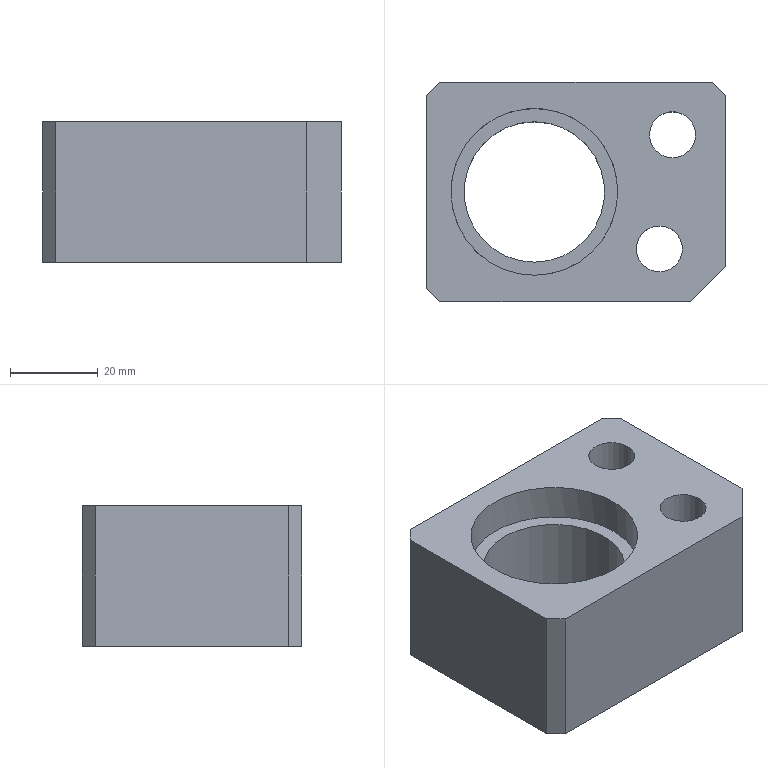Part | STEP file | lll_id3594_x_t | 1 solid | 19 faces | box 68 x 50 x 32 mm | volume 68588 mm3 | plane 13 | cylinder 6 | commonest cylinder face diameters 10.5 x2 17 x2 32 x1 38 x1
STEP:
#1=CARTESIAN_POINT('',(3231.727,69.288,77.5));
#2=VERTEX_POINT('',#1);
#3=CARTESIAN_POINT('',(3236.977,69.288,77.5));
#4=DIRECTION('',(0.,0.,1.));
#5=DIRECTION('',(-1.,0.,0.));
#6=AXIS2_PLACEMENT_3D('',#3,#4,#5);
#7=CIRCLE('',#6,5.25);
#8=EDGE_CURVE('',#2,#2,#7,.T.);
#9=ORIENTED_EDGE('',*,*,#8,.T.);
#10=EDGE_LOOP('',(#9));
#11=FACE_BOUND('',#10,.T.);
#12=CARTESIAN_POINT('',(3228.477,69.288,77.5));
#13=VERTEX_POINT('',#12);
#14=CARTESIAN_POINT('',(3236.977,69.288,77.5));
#15=DIRECTION('',(0.,0.,1.));
#16=DIRECTION('',(-1.,0.,0.));
#17=AXIS2_PLACEMENT_3D('',#14,#15,#16);
#18=CIRCLE('',#17,8.5);
#19=EDGE_CURVE('',#13,#13,#18,.T.);
#20=ORIENTED_EDGE('',*,*,#19,.F.);
#21=EDGE_LOOP('',(#20));
#22=FACE_BOUND('',#21,.T.);
#23=CARTESIAN_POINT('',(3236.977,69.288,77.5));
#24=DIRECTION('',(0.,0.,1.));
#25=DIRECTION('',(0.,1.,0.));
#26=AXIS2_PLACEMENT_3D('',#23,#24,#25);
#27=PLANE('',#26);
#28=ADVANCED_FACE('',(#11,#22),#27,.F.);
#29=CARTESIAN_POINT('',(3205.477,75.288,84.3));
#30=VERTEX_POINT('',#29);
#31=CARTESIAN_POINT('',(3205.477,56.288,84.3));
#32=DIRECTION('',(0.,0.,1.));
#33=DIRECTION('',(0.,1.,0.));
#34=AXIS2_PLACEMENT_3D('',#31,#32,#33);
#35=CIRCLE('',#34,19.);
#36=EDGE_CURVE('',#30,#30,#35,.T.);
#37=ORIENTED_EDGE('',*,*,#36,.T.);
#38=EDGE_LOOP('',(#37));
#39=FACE_BOUND('',#38,.T.);
#40=CARTESIAN_POINT('',(3205.477,72.288,84.3));
#41=VERTEX_POINT('',#40);
#42=CARTESIAN_POINT('',(3205.477,56.288,84.3));
#43=DIRECTION('',(0.,0.,1.));
#44=DIRECTION('',(0.,1.,0.));
#45=AXIS2_PLACEMENT_3D('',#42,#43,#44);
#46=CIRCLE('',#45,16.);
#47=EDGE_CURVE('',#41,#41,#46,.T.);
#48=ORIENTED_EDGE('',*,*,#47,.F.);
#49=EDGE_LOOP('',(#48));
#50=FACE_BOUND('',#49,.T.);
#51=CARTESIAN_POINT('',(3214.227,56.288,84.3));
#52=DIRECTION('',(0.,0.,-1.));
#53=DIRECTION('',(1.,0.,0.));
#54=AXIS2_PLACEMENT_3D('',#51,#52,#53);
#55=PLANE('',#54);
#56=ADVANCED_FACE('',(#39,#50),#55,.F.);
#57=ORIENTED_EDGE('',*,*,#19,.T.);
#58=EDGE_LOOP('',(#57));
#59=FACE_BOUND('',#58,.T.);
#60=CARTESIAN_POINT('',(3228.477,69.288,60.5));
#61=VERTEX_POINT('',#60);
#62=CARTESIAN_POINT('',(3236.977,69.288,60.5));
#63=DIRECTION('',(0.,0.,-1.));
#64=DIRECTION('',(-1.,0.,0.));
#65=AXIS2_PLACEMENT_3D('',#62,#63,#64);
#66=CIRCLE('',#65,8.5);
#67=EDGE_CURVE('',#61,#61,#66,.T.);
#68=ORIENTED_EDGE('',*,*,#67,.T.);
#69=EDGE_LOOP('',(#68));
#70=FACE_BOUND('',#69,.T.);
#71=CARTESIAN_POINT('',(3236.977,69.288,60.5));
#72=DIRECTION('',(0.,0.,1.));
#73=DIRECTION('',(0.,1.,0.));
#74=AXIS2_PLACEMENT_3D('',#71,#72,#73);
#75=CYLINDRICAL_SURFACE('',#74,8.5);
#76=ADVANCED_FACE('',(#59,#70),#75,.F.);
#77=CARTESIAN_POINT('',(3183.977,31.288,60.5));
#78=VERTEX_POINT('',#77);
#79=CARTESIAN_POINT('',(3180.977,34.288,60.5));
#80=VERTEX_POINT('',#79);
#81=CARTESIAN_POINT('',(3164.794,50.47,60.5));
#82=DIRECTION('',(-0.7071,0.7071,0.));
#83=VECTOR('',#82,1.);
#84=LINE('',#81,#83);
#85=EDGE_CURVE('',#78,#80,#84,.T.);
#86=ORIENTED_EDGE('',*,*,#85,.F.);
#87=CARTESIAN_POINT('',(3183.977,31.288,92.5));
#88=VERTEX_POINT('',#87);
#89=CARTESIAN_POINT('',(3183.977,31.288,-8.5));
#90=DIRECTION('',(0.,0.,-1.));
#91=VECTOR('',#90,1.);
#92=LINE('',#89,#91);
#93=EDGE_CURVE('',#88,#78,#92,.T.);
#94=ORIENTED_EDGE('',*,*,#93,.F.);
#95=CARTESIAN_POINT('',(3180.977,34.288,92.5));
#96=VERTEX_POINT('',#95);
#97=CARTESIAN_POINT('',(3164.794,50.47,92.5));
#98=DIRECTION('',(0.7071,-0.7071,0.));
#99=VECTOR('',#98,1.);
#100=LINE('',#97,#99);
#101=EDGE_CURVE('',#96,#88,#100,.T.);
#102=ORIENTED_EDGE('',*,*,#101,.F.);
#103=CARTESIAN_POINT('',(3180.977,34.288,-8.5));
#104=DIRECTION('',(0.,0.,1.));
#105=VECTOR('',#104,1.);
#106=LINE('',#103,#105);
#107=EDGE_CURVE('',#80,#96,#106,.T.);
#108=ORIENTED_EDGE('',*,*,#107,.F.);
#109=EDGE_LOOP('',(#86,#94,#102,#108));
#110=FACE_OUTER_BOUND('',#109,.T.);
#111=CARTESIAN_POINT('',(3180.977,34.288,-8.5));
#112=DIRECTION('',(0.7071,0.7071,0.));
#113=DIRECTION('',(0.,0.,1.));
#114=AXIS2_PLACEMENT_3D('',#111,#112,#113);
#115=PLANE('',#114);
#116=ADVANCED_FACE('',(#110),#115,.F.);
#117=CARTESIAN_POINT('',(3180.977,78.288,60.5));
#118=VERTEX_POINT('',#117);
#119=CARTESIAN_POINT('',(3180.977,119.478,60.5));
#120=DIRECTION('',(0.,1.,0.));
#121=VECTOR('',#120,1.);
#122=LINE('',#119,#121);
#123=EDGE_CURVE('',#80,#118,#122,.T.);
#124=ORIENTED_EDGE('',*,*,#123,.F.);
#125=ORIENTED_EDGE('',*,*,#107,.T.);
#126=CARTESIAN_POINT('',(3180.977,78.288,92.5));
#127=VERTEX_POINT('',#126);
#128=CARTESIAN_POINT('',(3180.977,56.288,92.5));
#129=DIRECTION('',(0.,-1.,0.));
#130=VECTOR('',#129,1.);
#131=LINE('',#128,#130);
#132=EDGE_CURVE('',#127,#96,#131,.T.);
#133=ORIENTED_EDGE('',*,*,#132,.F.);
#134=CARTESIAN_POINT('',(3180.977,78.288,-8.5));
#135=DIRECTION('',(0.,0.,1.));
#136=VECTOR('',#135,1.);
#137=LINE('',#134,#136);
#138=EDGE_CURVE('',#118,#127,#137,.T.);
#139=ORIENTED_EDGE('',*,*,#138,.F.);
#140=EDGE_LOOP('',(#124,#125,#133,#139));
#141=FACE_OUTER_BOUND('',#140,.T.);
#142=CARTESIAN_POINT('',(3180.977,56.288,-8.5));
#143=DIRECTION('',(-1.,0.,0.));
#144=DIRECTION('',(0.,0.,-1.));
#145=AXIS2_PLACEMENT_3D('',#142,#143,#144);
#146=PLANE('',#145);
#147=ADVANCED_FACE('',(#141),#146,.T.);
#148=CARTESIAN_POINT('',(3183.977,81.288,92.5));
#149=VERTEX_POINT('',#148);
#150=CARTESIAN_POINT('',(3183.977,81.288,92.5));
#151=DIRECTION('',(0.7071,0.7071,0.));
#152=VECTOR('',#151,1.);
#153=LINE('',#150,#152);
#154=EDGE_CURVE('',#127,#149,#153,.T.);
#155=ORIENTED_EDGE('',*,*,#154,.T.);
#156=CARTESIAN_POINT('',(3183.977,81.288,60.5));
#157=VERTEX_POINT('',#156);
#158=CARTESIAN_POINT('',(3183.977,81.288,-8.5));
#159=DIRECTION('',(0.,0.,-1.));
#160=VECTOR('',#159,1.);
#161=LINE('',#158,#160);
#162=EDGE_CURVE('',#149,#157,#161,.T.);
#163=ORIENTED_EDGE('',*,*,#162,.T.);
#164=CARTESIAN_POINT('',(3179.027,76.338,60.5));
#165=DIRECTION('',(-0.7071,-0.7071,0.));
#166=VECTOR('',#165,1.);
#167=LINE('',#164,#166);
#168=EDGE_CURVE('',#157,#118,#167,.T.);
#169=ORIENTED_EDGE('',*,*,#168,.T.);
#170=ORIENTED_EDGE('',*,*,#138,.T.);
#171=EDGE_LOOP('',(#155,#163,#169,#170));
#172=FACE_OUTER_BOUND('',#171,.T.);
#173=CARTESIAN_POINT('',(3183.977,81.288,-8.5));
#174=DIRECTION('',(0.7071,-0.7071,0.));
#175=DIRECTION('',(0.7071,0.7071,0.));
#176=AXIS2_PLACEMENT_3D('',#173,#174,#175);
#177=PLANE('',#176);
#178=ADVANCED_FACE('',(#172),#177,.F.);
#179=CARTESIAN_POINT('',(3245.977,81.288,60.5));
#180=VERTEX_POINT('',#179);
#181=CARTESIAN_POINT('',(3231.752,81.288,60.5));
#182=DIRECTION('',(1.,0.,0.));
#183=VECTOR('',#182,1.);
#184=LINE('',#181,#183);
#185=EDGE_CURVE('',#157,#180,#184,.T.);
#186=ORIENTED_EDGE('',*,*,#185,.F.);
#187=ORIENTED_EDGE('',*,*,#162,.F.);
#188=CARTESIAN_POINT('',(3245.977,81.288,92.5));
#189=VERTEX_POINT('',#188);
#190=CARTESIAN_POINT('',(3236.702,81.288,92.5));
#191=DIRECTION('',(-1.,0.,0.));
#192=VECTOR('',#191,1.);
#193=LINE('',#190,#192);
#194=EDGE_CURVE('',#189,#149,#193,.T.);
#195=ORIENTED_EDGE('',*,*,#194,.F.);
#196=CARTESIAN_POINT('',(3245.977,81.288,-8.5));
#197=DIRECTION('',(0.,0.,1.));
#198=VECTOR('',#197,1.);
#199=LINE('',#196,#198);
#200=EDGE_CURVE('',#180,#189,#199,.T.);
#201=ORIENTED_EDGE('',*,*,#200,.F.);
#202=EDGE_LOOP('',(#186,#187,#195,#201));
#203=FACE_OUTER_BOUND('',#202,.T.);
#204=CARTESIAN_POINT('',(3205.477,81.288,-8.5));
#205=DIRECTION('',(0.,1.,0.));
#206=DIRECTION('',(0.,0.,-1.));
#207=AXIS2_PLACEMENT_3D('',#204,#205,#206);
#208=PLANE('',#207);
#209=ADVANCED_FACE('',(#203),#208,.T.);
#210=CARTESIAN_POINT('',(3248.977,78.288,92.5));
#211=VERTEX_POINT('',#210);
#212=CARTESIAN_POINT('',(3248.977,78.288,92.5));
#213=DIRECTION('',(0.7071,-0.7071,0.));
#214=VECTOR('',#213,1.);
#215=LINE('',#212,#214);
#216=EDGE_CURVE('',#189,#211,#215,.T.);
#217=ORIENTED_EDGE('',*,*,#216,.T.);
#218=CARTESIAN_POINT('',(3248.977,78.288,60.5));
#219=VERTEX_POINT('',#218);
#220=CARTESIAN_POINT('',(3248.977,78.288,-8.5));
#221=DIRECTION('',(0.,0.,-1.));
#222=VECTOR('',#221,1.);
#223=LINE('',#220,#222);
#224=EDGE_CURVE('',#211,#219,#223,.T.);
#225=ORIENTED_EDGE('',*,*,#224,.T.);
#226=CARTESIAN_POINT('',(3248.977,78.288,60.5));
#227=DIRECTION('',(-0.7071,0.7071,0.));
#228=VECTOR('',#227,1.);
#229=LINE('',#226,#228);
#230=EDGE_CURVE('',#219,#180,#229,.T.);
#231=ORIENTED_EDGE('',*,*,#230,.T.);
#232=ORIENTED_EDGE('',*,*,#200,.T.);
#233=EDGE_LOOP('',(#217,#225,#231,#232));
#234=FACE_OUTER_BOUND('',#233,.T.);
#235=CARTESIAN_POINT('',(3248.977,78.288,-8.5));
#236=DIRECTION('',(-0.7071,-0.7071,0.));
#237=DIRECTION('',(0.7071,-0.7071,0.));
#238=AXIS2_PLACEMENT_3D('',#235,#236,#237);
#239=PLANE('',#238);
#240=ADVANCED_FACE('',(#234),#239,.F.);
#241=CARTESIAN_POINT('',(3248.977,39.288,92.5));
#242=VERTEX_POINT('',#241);
#243=CARTESIAN_POINT('',(3248.977,56.288,92.5));
#244=DIRECTION('',(0.,1.,0.));
#245=VECTOR('',#244,1.);
#246=LINE('',#243,#245);
#247=EDGE_CURVE('',#242,#211,#246,.T.);
#248=ORIENTED_EDGE('',*,*,#247,.F.);
#249=CARTESIAN_POINT('',(3248.977,39.288,60.5));
#250=VERTEX_POINT('',#249);
#251=CARTESIAN_POINT('',(3248.977,39.288,-8.5));
#252=DIRECTION('',(0.,0.,-1.));
#253=VECTOR('',#252,1.);
#254=LINE('',#251,#253);
#255=EDGE_CURVE('',#242,#250,#254,.T.);
#256=ORIENTED_EDGE('',*,*,#255,.T.);
#257=CARTESIAN_POINT('',(3248.977,119.478,60.5));
#258=DIRECTION('',(0.,-1.,0.));
#259=VECTOR('',#258,1.);
#260=LINE('',#257,#259);
#261=EDGE_CURVE('',#219,#250,#260,.T.);
#262=ORIENTED_EDGE('',*,*,#261,.F.);
#263=ORIENTED_EDGE('',*,*,#224,.F.);
#264=EDGE_LOOP('',(#248,#256,#262,#263));
#265=FACE_OUTER_BOUND('',#264,.T.);
#266=CARTESIAN_POINT('',(3248.977,56.288,-8.5));
#267=DIRECTION('',(1.,0.,0.));
#268=DIRECTION('',(0.,0.,1.));
#269=AXIS2_PLACEMENT_3D('',#266,#267,#268);
#270=PLANE('',#269);
#271=ADVANCED_FACE('',(#265),#270,.T.);
#272=CARTESIAN_POINT('',(3240.977,31.288,92.5));
#273=VERTEX_POINT('',#272);
#274=CARTESIAN_POINT('',(3284.384,74.696,92.5));
#275=DIRECTION('',(0.7071,0.7071,0.));
#276=VECTOR('',#275,1.);
#277=LINE('',#274,#276);
#278=EDGE_CURVE('',#273,#242,#277,.T.);
#279=ORIENTED_EDGE('',*,*,#278,.F.);
#280=CARTESIAN_POINT('',(3240.977,31.288,60.5));
#281=VERTEX_POINT('',#280);
#282=CARTESIAN_POINT('',(3240.977,31.288,-8.5));
#283=DIRECTION('',(0.,0.,1.));
#284=VECTOR('',#283,1.);
#285=LINE('',#282,#284);
#286=EDGE_CURVE('',#281,#273,#285,.T.);
#287=ORIENTED_EDGE('',*,*,#286,.F.);
#288=CARTESIAN_POINT('',(3279.434,69.746,60.5));
#289=DIRECTION('',(-0.7071,-0.7071,0.));
#290=VECTOR('',#289,1.);
#291=LINE('',#288,#290);
#292=EDGE_CURVE('',#250,#281,#291,.T.);
#293=ORIENTED_EDGE('',*,*,#292,.F.);
#294=ORIENTED_EDGE('',*,*,#255,.F.);
#295=EDGE_LOOP('',(#279,#287,#293,#294));
#296=FACE_OUTER_BOUND('',#295,.T.);
#297=CARTESIAN_POINT('',(3248.977,39.288,-8.5));
#298=DIRECTION('',(-0.7071,0.7071,0.));
#299=DIRECTION('',(0.,0.,-1.));
#300=AXIS2_PLACEMENT_3D('',#297,#298,#299);
#301=PLANE('',#300);
#302=ADVANCED_FACE('',(#296),#301,.F.);
#303=CARTESIAN_POINT('',(3231.752,31.288,60.5));
#304=DIRECTION('',(-1.,0.,0.));
#305=VECTOR('',#304,1.);
#306=LINE('',#303,#305);
#307=EDGE_CURVE('',#281,#78,#306,.T.);
#308=ORIENTED_EDGE('',*,*,#307,.F.);
#309=ORIENTED_EDGE('',*,*,#286,.T.);
#310=CARTESIAN_POINT('',(3231.752,31.288,92.5));
#311=DIRECTION('',(1.,0.,0.));
#312=VECTOR('',#311,1.);
#313=LINE('',#310,#312);
#314=EDGE_CURVE('',#88,#273,#313,.T.);
#315=ORIENTED_EDGE('',*,*,#314,.F.);
#316=ORIENTED_EDGE('',*,*,#93,.T.);
#317=EDGE_LOOP('',(#308,#309,#315,#316));
#318=FACE_OUTER_BOUND('',#317,.T.);
#319=CARTESIAN_POINT('',(3200.527,31.288,-8.5));
#320=DIRECTION('',(0.,-1.,0.));
#321=DIRECTION('',(0.,0.,1.));
#322=AXIS2_PLACEMENT_3D('',#319,#320,#321);
#323=PLANE('',#322);
#324=ADVANCED_FACE('',(#318),#323,.T.);
#325=CARTESIAN_POINT('',(3231.727,69.288,92.5));
#326=VERTEX_POINT('',#325);
#327=CARTESIAN_POINT('',(3236.977,69.288,92.5));
#328=DIRECTION('',(0.,0.,-1.));
#329=DIRECTION('',(-1.,0.,0.));
#330=AXIS2_PLACEMENT_3D('',#327,#328,#329);
#331=CIRCLE('',#330,5.25);
#332=EDGE_CURVE('',#326,#326,#331,.T.);
#333=ORIENTED_EDGE('',*,*,#332,.F.);
#334=EDGE_LOOP('',(#333));
#335=FACE_BOUND('',#334,.T.);
#336=ORIENTED_EDGE('',*,*,#8,.F.);
#337=EDGE_LOOP('',(#336));
#338=FACE_BOUND('',#337,.T.);
#339=CARTESIAN_POINT('',(3236.977,69.288,160.5));
#340=DIRECTION('',(0.,0.,1.));
#341=DIRECTION('',(0.,1.,0.));
#342=AXIS2_PLACEMENT_3D('',#339,#340,#341);
#343=CYLINDRICAL_SURFACE('',#342,5.25);
#344=ADVANCED_FACE('',(#335,#338),#343,.F.);
#345=CARTESIAN_POINT('',(3205.477,37.288,92.5));
#346=VERTEX_POINT('',#345);
#347=CARTESIAN_POINT('',(3205.477,56.288,92.5));
#348=DIRECTION('',(0.,0.,-1.));
#349=DIRECTION('',(0.,-1.,0.));
#350=AXIS2_PLACEMENT_3D('',#347,#348,#349);
#351=CIRCLE('',#350,19.);
#352=EDGE_CURVE('',#346,#346,#351,.T.);
#353=ORIENTED_EDGE('',*,*,#352,.F.);
#354=EDGE_LOOP('',(#353));
#355=FACE_BOUND('',#354,.T.);
#356=ORIENTED_EDGE('',*,*,#36,.F.);
#357=EDGE_LOOP('',(#356));
#358=FACE_BOUND('',#357,.T.);
#359=CARTESIAN_POINT('',(3205.477,56.288,90.));
#360=DIRECTION('',(0.,0.,-1.));
#361=DIRECTION('',(-1.,0.,0.));
#362=AXIS2_PLACEMENT_3D('',#359,#360,#361);
#363=CYLINDRICAL_SURFACE('',#362,19.);
#364=ADVANCED_FACE('',(#355,#358),#363,.F.);
#365=CARTESIAN_POINT('',(3239.227,43.288,92.5));
#366=VERTEX_POINT('',#365);
#367=CARTESIAN_POINT('',(3233.977,43.288,92.5));
#368=DIRECTION('',(0.,0.,1.));
#369=DIRECTION('',(1.,0.,0.));
#370=AXIS2_PLACEMENT_3D('',#367,#368,#369);
#371=CIRCLE('',#370,5.25);
#372=EDGE_CURVE('',#366,#366,#371,.T.);
#373=ORIENTED_EDGE('',*,*,#372,.F.);
#374=EDGE_LOOP('',(#373));
#375=FACE_BOUND('',#374,.T.);
#376=ORIENTED_EDGE('',*,*,#352,.T.);
#377=EDGE_LOOP('',(#376));
#378=FACE_BOUND('',#377,.T.);
#379=ORIENTED_EDGE('',*,*,#332,.T.);
#380=EDGE_LOOP('',(#379));
#381=FACE_BOUND('',#380,.T.);
#382=ORIENTED_EDGE('',*,*,#314,.T.);
#383=ORIENTED_EDGE('',*,*,#278,.T.);
#384=ORIENTED_EDGE('',*,*,#247,.T.);
#385=ORIENTED_EDGE('',*,*,#216,.F.);
#386=ORIENTED_EDGE('',*,*,#194,.T.);
#387=ORIENTED_EDGE('',*,*,#154,.F.);
#388=ORIENTED_EDGE('',*,*,#132,.T.);
#389=ORIENTED_EDGE('',*,*,#101,.T.);
#390=EDGE_LOOP('',(#382,#383,#384,#385,#386,#387,#388,#389));
#391=FACE_BOUND('',#390,.T.);
#392=CARTESIAN_POINT('',(3236.702,124.428,92.5));
#393=DIRECTION('',(0.,0.,1.));
#394=DIRECTION('',(0.,1.,0.));
#395=AXIS2_PLACEMENT_3D('',#392,#393,#394);
#396=PLANE('',#395);
#397=ADVANCED_FACE('',(#375,#378,#381,#391),#396,.T.);
#398=CARTESIAN_POINT('',(3205.477,40.288,60.5));
#399=VERTEX_POINT('',#398);
#400=CARTESIAN_POINT('',(3205.477,56.288,60.5));
#401=DIRECTION('',(0.,0.,1.));
#402=DIRECTION('',(0.,-1.,0.));
#403=AXIS2_PLACEMENT_3D('',#400,#401,#402);
#404=CIRCLE('',#403,16.);
#405=EDGE_CURVE('',#399,#399,#404,.T.);
#406=ORIENTED_EDGE('',*,*,#405,.F.);
#407=EDGE_LOOP('',(#406));
#408=FACE_BOUND('',#407,.T.);
#409=ORIENTED_EDGE('',*,*,#47,.T.);
#410=EDGE_LOOP('',(#409));
#411=FACE_BOUND('',#410,.T.);
#412=CARTESIAN_POINT('',(3205.477,56.288,44.8));
#413=DIRECTION('',(0.,0.,-1.));
#414=DIRECTION('',(-1.,0.,0.));
#415=AXIS2_PLACEMENT_3D('',#412,#413,#414);
#416=CYLINDRICAL_SURFACE('',#415,16.);
#417=ADVANCED_FACE('',(#408,#411),#416,.F.);
#418=CARTESIAN_POINT('',(3242.477,43.288,60.5));
#419=VERTEX_POINT('',#418);
#420=CARTESIAN_POINT('',(3233.977,43.288,60.5));
#421=DIRECTION('',(0.,0.,-1.));
#422=DIRECTION('',(1.,0.,0.));
#423=AXIS2_PLACEMENT_3D('',#420,#421,#422);
#424=CIRCLE('',#423,8.5);
#425=EDGE_CURVE('',#419,#419,#424,.T.);
#426=ORIENTED_EDGE('',*,*,#425,.F.);
#427=EDGE_LOOP('',(#426));
#428=FACE_BOUND('',#427,.T.);
#429=ORIENTED_EDGE('',*,*,#405,.T.);
#430=EDGE_LOOP('',(#429));
#431=FACE_BOUND('',#430,.T.);
#432=ORIENTED_EDGE('',*,*,#261,.T.);
#433=ORIENTED_EDGE('',*,*,#292,.T.);
#434=ORIENTED_EDGE('',*,*,#307,.T.);
#435=ORIENTED_EDGE('',*,*,#85,.T.);
#436=ORIENTED_EDGE('',*,*,#123,.T.);
#437=ORIENTED_EDGE('',*,*,#168,.F.);
#438=ORIENTED_EDGE('',*,*,#185,.T.);
#439=ORIENTED_EDGE('',*,*,#230,.F.);
#440=EDGE_LOOP('',(#432,#433,#434,#435,#436,#437,#438,#439));
#441=FACE_BOUND('',#440,.T.);
#442=ORIENTED_EDGE('',*,*,#67,.F.);
#443=EDGE_LOOP('',(#442));
#444=FACE_BOUND('',#443,.T.);
#445=CARTESIAN_POINT('',(3231.752,119.478,60.5));
#446=DIRECTION('',(0.,0.,1.));
#447=DIRECTION('',(0.,1.,0.));
#448=AXIS2_PLACEMENT_3D('',#445,#446,#447);
#449=PLANE('',#448);
#450=ADVANCED_FACE('',(#428,#431,#441,#444),#449,.F.);
#451=CARTESIAN_POINT('',(3228.727,43.288,77.5));
#452=VERTEX_POINT('',#451);
#453=CARTESIAN_POINT('',(3233.977,43.288,77.5));
#454=DIRECTION('',(0.,0.,1.));
#455=DIRECTION('',(-1.,0.,0.));
#456=AXIS2_PLACEMENT_3D('',#453,#454,#455);
#457=CIRCLE('',#456,5.25);
#458=EDGE_CURVE('',#452,#452,#457,.T.);
#459=ORIENTED_EDGE('',*,*,#458,.T.);
#460=EDGE_LOOP('',(#459));
#461=FACE_BOUND('',#460,.T.);
#462=CARTESIAN_POINT('',(3225.477,43.288,77.5));
#463=VERTEX_POINT('',#462);
#464=CARTESIAN_POINT('',(3233.977,43.288,77.5));
#465=DIRECTION('',(0.,0.,1.));
#466=DIRECTION('',(-1.,0.,0.));
#467=AXIS2_PLACEMENT_3D('',#464,#465,#466);
#468=CIRCLE('',#467,8.5);
#469=EDGE_CURVE('',#463,#463,#468,.T.);
#470=ORIENTED_EDGE('',*,*,#469,.F.);
#471=EDGE_LOOP('',(#470));
#472=FACE_BOUND('',#471,.T.);
#473=CARTESIAN_POINT('',(3236.977,43.288,77.5));
#474=DIRECTION('',(0.,0.,1.));
#475=DIRECTION('',(0.,-1.,0.));
#476=AXIS2_PLACEMENT_3D('',#473,#474,#475);
#477=PLANE('',#476);
#478=ADVANCED_FACE('',(#461,#472),#477,.F.);
#479=ORIENTED_EDGE('',*,*,#372,.T.);
#480=EDGE_LOOP('',(#479));
#481=FACE_BOUND('',#480,.T.);
#482=ORIENTED_EDGE('',*,*,#458,.F.);
#483=EDGE_LOOP('',(#482));
#484=FACE_BOUND('',#483,.T.);
#485=CARTESIAN_POINT('',(3233.977,43.288,160.5));
#486=DIRECTION('',(0.,0.,1.));
#487=DIRECTION('',(0.,-1.,0.));
#488=AXIS2_PLACEMENT_3D('',#485,#486,#487);
#489=CYLINDRICAL_SURFACE('',#488,5.25);
#490=ADVANCED_FACE('',(#481,#484),#489,.F.);
#491=ORIENTED_EDGE('',*,*,#469,.T.);
#492=EDGE_LOOP('',(#491));
#493=FACE_BOUND('',#492,.T.);
#494=ORIENTED_EDGE('',*,*,#425,.T.);
#495=EDGE_LOOP('',(#494));
#496=FACE_BOUND('',#495,.T.);
#497=CARTESIAN_POINT('',(3233.977,43.288,60.5));
#498=DIRECTION('',(0.,0.,1.));
#499=DIRECTION('',(0.,-1.,0.));
#500=AXIS2_PLACEMENT_3D('',#497,#498,#499);
#501=CYLINDRICAL_SURFACE('',#500,8.5);
#502=ADVANCED_FACE('',(#493,#496),#501,.F.);
#503=CLOSED_SHELL('',(#28,#56,#76,#116,#147,#178,#209,#240,#271,#302,#324,#344,#364,#397,#417,#450,#478,#490,#502));
#504=MANIFOLD_SOLID_BREP('',#503);
#505=(LENGTH_UNIT()NAMED_UNIT(*)SI_UNIT(.MILLI.,.METRE.));
#506=UNCERTAINTY_MEASURE_WITH_UNIT(LENGTH_MEASURE(0.00002),#505,'','');
#507=(NAMED_UNIT(*)PLANE_ANGLE_UNIT()SI_UNIT($,.RADIAN.));
#508=PLANE_ANGLE_MEASURE_WITH_UNIT(PLANE_ANGLE_MEASURE(0.01745),#507);
#509=DIMENSIONAL_EXPONENTS(0.,0.,0.,0.,0.,0.,0.);
#510=(CONVERSION_BASED_UNIT('DEGREE',#508)NAMED_UNIT(#509)PLANE_ANGLE_UNIT());
#511=(NAMED_UNIT(*)SI_UNIT($,.STERADIAN.)SOLID_ANGLE_UNIT());
#512=(GEOMETRIC_REPRESENTATION_CONTEXT(3)GLOBAL_UNCERTAINTY_ASSIGNED_CONTEXT((#506))GLOBAL_UNIT_ASSIGNED_CONTEXT((#505,#510,#511))REPRESENTATION_CONTEXT('',''));
#513=ADVANCED_BREP_SHAPE_REPRESENTATION('',(#504),#512);